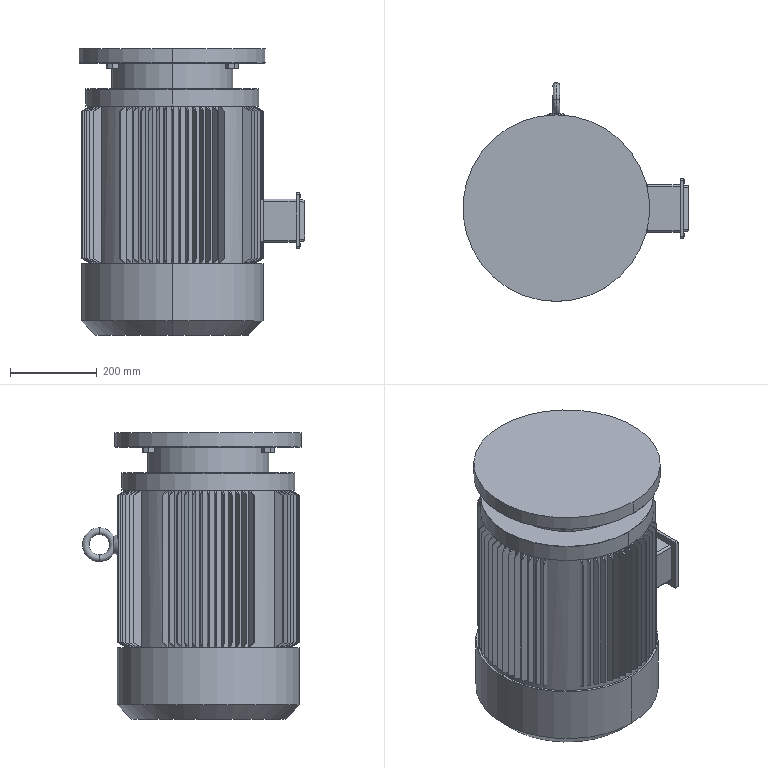Part | SolidWorks | features BaseBody 2 | 2 solids | 550 faces | box 520 x 505.12 x 660 mm | volume 80018411 mm3 | plane 381 | cylinder 121 | cone 40 | spline 4 | torus 4 | commonest cylinder face diameters 420 x63 4.455 x20 8.91 x12 7.425 x8 378 x6 3.319 x4